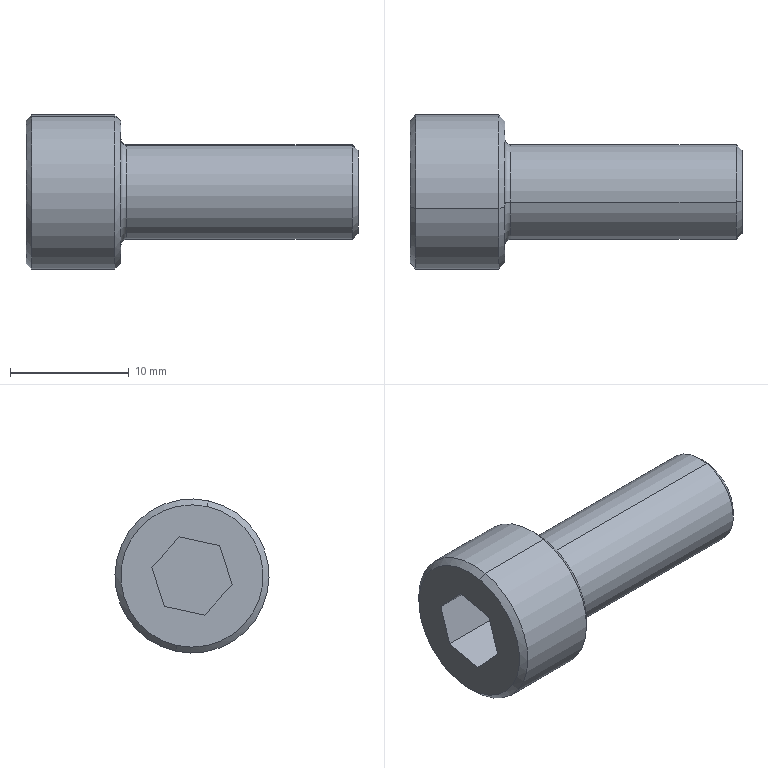Part | NX | features BREP 1 | 1 solid | 22 faces | box 28 x 13 x 13 mm | volume 1869 mm3 | plane 10 | cone 6 | cylinder 4 | torus 2 | commonest cylinder face diameters 8 x2 13 x2
STEP:
#1=CARTESIAN_POINT('',(-655.355,-109.755,15.547));
#2=VERTEX_POINT('',#1);
#3=CARTESIAN_POINT('',(-655.355,-111.682,24.338));
#4=VERTEX_POINT('',#3);
#5=CARTESIAN_POINT('',(-655.355,-110.718,19.942));
#6=DIRECTION('',(-1.,0.,0.));
#7=DIRECTION('',(0.,-0.2141,0.9768));
#8=AXIS2_PLACEMENT_3D('',#5,#6,#7);
#9=CIRCLE('',#8,4.5);
#10=EDGE_CURVE('',#2,#4,#9,.T.);
#11=ORIENTED_EDGE('',*,*,#10,.F.);
#12=CARTESIAN_POINT('',(-654.855,-109.862,16.035));
#13=VERTEX_POINT('',#12);
#14=CARTESIAN_POINT('',(-654.855,-109.755,15.547));
#15=DIRECTION('',(0.,0.9768,0.2141));
#16=DIRECTION('',(0.,0.2141,-0.9768));
#17=AXIS2_PLACEMENT_3D('',#14,#15,#16);
#18=CIRCLE('',#17,0.5);
#19=EDGE_CURVE('',#13,#2,#18,.F.);
#20=ORIENTED_EDGE('',*,*,#19,.F.);
#21=CARTESIAN_POINT('',(-654.855,-111.575,23.85));
#22=VERTEX_POINT('',#21);
#23=CARTESIAN_POINT('',(-654.855,-110.718,19.942));
#24=DIRECTION('',(1.,0.,0.));
#25=DIRECTION('',(0.,-0.2141,0.9768));
#26=AXIS2_PLACEMENT_3D('',#23,#24,#25);
#27=CIRCLE('',#26,4.);
#28=EDGE_CURVE('',#22,#13,#27,.T.);
#29=ORIENTED_EDGE('',*,*,#28,.F.);
#30=CARTESIAN_POINT('',(-654.855,-111.682,24.338));
#31=DIRECTION('',(0.,-0.9768,-0.2141));
#32=DIRECTION('',(1.,0.,0.));
#33=AXIS2_PLACEMENT_3D('',#30,#31,#32);
#34=CIRCLE('',#33,0.5);
#35=EDGE_CURVE('',#22,#4,#34,.F.);
#36=ORIENTED_EDGE('',*,*,#35,.T.);
#37=EDGE_LOOP('',(#11,#20,#29,#36));
#38=FACE_BOUND('',#37,.T.);
#39=CARTESIAN_POINT('',(-654.855,-110.718,19.942));
#40=DIRECTION('',(-1.,0.,0.));
#41=DIRECTION('',(0.,-0.2141,0.9768));
#42=AXIS2_PLACEMENT_3D('',#39,#40,#41);
#43=TOROIDAL_SURFACE('',#42,4.5,0.5);
#44=ADVANCED_FACE('',(#38),#43,.F.);
#45=CARTESIAN_POINT('',(-635.355,-109.969,16.524));
#46=VERTEX_POINT('',#45);
#47=CARTESIAN_POINT('',(-635.355,-111.468,23.361));
#48=VERTEX_POINT('',#47);
#49=CARTESIAN_POINT('',(-635.355,-110.718,19.942));
#50=DIRECTION('',(1.,0.,0.));
#51=DIRECTION('',(0.,-0.2141,0.9768));
#52=AXIS2_PLACEMENT_3D('',#49,#50,#51);
#53=CIRCLE('',#52,3.5);
#54=EDGE_CURVE('',#46,#48,#53,.T.);
#55=ORIENTED_EDGE('',*,*,#54,.F.);
#56=CARTESIAN_POINT('',(-635.855,-109.862,16.035));
#57=VERTEX_POINT('',#56);
#58=CARTESIAN_POINT('',(-635.855,-109.862,16.035));
#59=DIRECTION('',(-0.7071,0.1514,-0.6907));
#60=VECTOR('',#59,1000.);
#61=LINE('',#58,#60);
#62=EDGE_CURVE('',#57,#46,#61,.F.);
#63=ORIENTED_EDGE('',*,*,#62,.F.);
#64=CARTESIAN_POINT('',(-635.855,-111.575,23.85));
#65=VERTEX_POINT('',#64);
#66=CARTESIAN_POINT('',(-635.855,-110.718,19.942));
#67=DIRECTION('',(-1.,0.,0.));
#68=DIRECTION('',(0.,-0.2141,0.9768));
#69=AXIS2_PLACEMENT_3D('',#66,#67,#68);
#70=CIRCLE('',#69,4.);
#71=EDGE_CURVE('',#65,#57,#70,.T.);
#72=ORIENTED_EDGE('',*,*,#71,.F.);
#73=CARTESIAN_POINT('',(-635.855,-111.575,23.85));
#74=DIRECTION('',(-0.7071,-0.1514,0.6907));
#75=VECTOR('',#74,1000.);
#76=LINE('',#73,#75);
#77=EDGE_CURVE('',#65,#48,#76,.F.);
#78=ORIENTED_EDGE('',*,*,#77,.T.);
#79=EDGE_LOOP('',(#55,#63,#72,#78));
#80=FACE_BOUND('',#79,.T.);
#81=CARTESIAN_POINT('',(-635.855,-110.718,19.942));
#82=DIRECTION('',(-1.,0.,0.));
#83=DIRECTION('',(0.,-0.2141,0.9768));
#84=AXIS2_PLACEMENT_3D('',#81,#82,#83);
#85=CONICAL_SURFACE('',#84,4.,0.7854);
#86=ADVANCED_FACE('',(#80),#85,.T.);
#87=CARTESIAN_POINT('',(-663.355,-112.003,25.803));
#88=VERTEX_POINT('',#87);
#89=CARTESIAN_POINT('',(-663.355,-109.434,14.082));
#90=VERTEX_POINT('',#89);
#91=CARTESIAN_POINT('',(-663.355,-110.718,19.942));
#92=DIRECTION('',(-1.,0.,0.));
#93=DIRECTION('',(0.,-0.2141,0.9768));
#94=AXIS2_PLACEMENT_3D('',#91,#92,#93);
#95=CIRCLE('',#94,6.);
#96=EDGE_CURVE('',#88,#90,#95,.T.);
#97=ORIENTED_EDGE('',*,*,#96,.F.);
#98=CARTESIAN_POINT('',(-662.855,-112.11,26.292));
#99=VERTEX_POINT('',#98);
#100=CARTESIAN_POINT('',(-663.355,-112.003,25.803));
#101=DIRECTION('',(0.7071,-0.1514,0.6907));
#102=VECTOR('',#101,1000.);
#103=LINE('',#100,#102);
#104=EDGE_CURVE('',#88,#99,#103,.T.);
#105=ORIENTED_EDGE('',*,*,#104,.T.);
#106=CARTESIAN_POINT('',(-662.855,-109.326,13.593));
#107=VERTEX_POINT('',#106);
#108=CARTESIAN_POINT('',(-662.855,-110.718,19.942));
#109=DIRECTION('',(1.,0.,0.));
#110=DIRECTION('',(0.,-0.2141,0.9768));
#111=AXIS2_PLACEMENT_3D('',#108,#109,#110);
#112=CIRCLE('',#111,6.5);
#113=EDGE_CURVE('',#107,#99,#112,.T.);
#114=ORIENTED_EDGE('',*,*,#113,.F.);
#115=CARTESIAN_POINT('',(-663.355,-109.434,14.082));
#116=DIRECTION('',(0.7071,0.1514,-0.6907));
#117=VECTOR('',#116,1000.);
#118=LINE('',#115,#117);
#119=EDGE_CURVE('',#90,#107,#118,.T.);
#120=ORIENTED_EDGE('',*,*,#119,.F.);
#121=EDGE_LOOP('',(#97,#105,#114,#120));
#122=FACE_BOUND('',#121,.T.);
#123=CARTESIAN_POINT('',(-663.355,-110.718,19.942));
#124=DIRECTION('',(1.,0.,0.));
#125=DIRECTION('',(0.,0.2141,-0.9768));
#126=AXIS2_PLACEMENT_3D('',#123,#124,#125);
#127=CONICAL_SURFACE('',#126,6.,0.7854);
#128=ADVANCED_FACE('',(#122),#127,.T.);
#129=CARTESIAN_POINT('',(-655.355,-109.434,14.082));
#130=VERTEX_POINT('',#129);
#131=CARTESIAN_POINT('',(-655.355,-112.003,25.803));
#132=VERTEX_POINT('',#131);
#133=CARTESIAN_POINT('',(-655.355,-110.718,19.942));
#134=DIRECTION('',(1.,0.,0.));
#135=DIRECTION('',(0.,-0.2141,0.9768));
#136=AXIS2_PLACEMENT_3D('',#133,#134,#135);
#137=CIRCLE('',#136,6.);
#138=EDGE_CURVE('',#130,#132,#137,.T.);
#139=ORIENTED_EDGE('',*,*,#138,.F.);
#140=CARTESIAN_POINT('',(-655.855,-109.326,13.593));
#141=VERTEX_POINT('',#140);
#142=CARTESIAN_POINT('',(-655.855,-109.326,13.593));
#143=DIRECTION('',(-0.7071,0.1514,-0.6907));
#144=VECTOR('',#143,1000.);
#145=LINE('',#142,#144);
#146=EDGE_CURVE('',#141,#130,#145,.F.);
#147=ORIENTED_EDGE('',*,*,#146,.F.);
#148=CARTESIAN_POINT('',(-655.855,-112.11,26.292));
#149=VERTEX_POINT('',#148);
#150=CARTESIAN_POINT('',(-655.855,-110.718,19.942));
#151=DIRECTION('',(-1.,0.,0.));
#152=DIRECTION('',(0.,-0.2141,0.9768));
#153=AXIS2_PLACEMENT_3D('',#150,#151,#152);
#154=CIRCLE('',#153,6.5);
#155=EDGE_CURVE('',#149,#141,#154,.T.);
#156=ORIENTED_EDGE('',*,*,#155,.F.);
#157=CARTESIAN_POINT('',(-655.855,-112.11,26.292));
#158=DIRECTION('',(-0.7071,-0.1514,0.6907));
#159=VECTOR('',#158,1000.);
#160=LINE('',#157,#159);
#161=EDGE_CURVE('',#149,#132,#160,.F.);
#162=ORIENTED_EDGE('',*,*,#161,.T.);
#163=EDGE_LOOP('',(#139,#147,#156,#162));
#164=FACE_BOUND('',#163,.T.);
#165=CARTESIAN_POINT('',(-655.855,-110.718,19.942));
#166=DIRECTION('',(-1.,0.,0.));
#167=DIRECTION('',(0.,-0.2141,0.9768));
#168=AXIS2_PLACEMENT_3D('',#165,#166,#167);
#169=CONICAL_SURFACE('',#168,6.5,0.7854);
#170=ADVANCED_FACE('',(#164),#169,.T.);
#171=ORIENTED_EDGE('',*,*,#113,.T.);
#172=CARTESIAN_POINT('',(-663.355,-112.11,26.292));
#173=DIRECTION('',(1.,0.,0.));
#174=VECTOR('',#173,1000.);
#175=LINE('',#172,#174);
#176=EDGE_CURVE('',#99,#149,#175,.T.);
#177=ORIENTED_EDGE('',*,*,#176,.T.);
#178=ORIENTED_EDGE('',*,*,#155,.T.);
#179=CARTESIAN_POINT('',(-663.355,-109.326,13.593));
#180=DIRECTION('',(1.,0.,0.));
#181=VECTOR('',#180,1000.);
#182=LINE('',#179,#181);
#183=EDGE_CURVE('',#107,#141,#182,.T.);
#184=ORIENTED_EDGE('',*,*,#183,.F.);
#185=EDGE_LOOP('',(#171,#177,#178,#184));
#186=FACE_BOUND('',#185,.T.);
#187=CARTESIAN_POINT('',(-663.355,-110.718,19.942));
#188=DIRECTION('',(1.,0.,0.));
#189=DIRECTION('',(0.,0.2141,-0.9768));
#190=AXIS2_PLACEMENT_3D('',#187,#188,#189);
#191=CYLINDRICAL_SURFACE('',#190,6.5);
#192=ADVANCED_FACE('',(#186),#191,.T.);
#193=CARTESIAN_POINT('',(-654.855,-110.718,19.942));
#194=DIRECTION('',(1.,0.,0.));
#195=DIRECTION('',(0.,-0.2141,0.9768));
#196=AXIS2_PLACEMENT_3D('',#193,#194,#195);
#197=CIRCLE('',#196,4.);
#198=EDGE_CURVE('',#13,#22,#197,.T.);
#199=ORIENTED_EDGE('',*,*,#198,.T.);
#200=CARTESIAN_POINT('',(-655.355,-111.575,23.85));
#201=DIRECTION('',(1.,0.,0.));
#202=VECTOR('',#201,1000.);
#203=LINE('',#200,#202);
#204=EDGE_CURVE('',#22,#65,#203,.T.);
#205=ORIENTED_EDGE('',*,*,#204,.T.);
#206=ORIENTED_EDGE('',*,*,#71,.T.);
#207=CARTESIAN_POINT('',(-655.355,-109.862,16.035));
#208=DIRECTION('',(1.,0.,0.));
#209=VECTOR('',#208,1000.);
#210=LINE('',#207,#209);
#211=EDGE_CURVE('',#13,#57,#210,.T.);
#212=ORIENTED_EDGE('',*,*,#211,.F.);
#213=EDGE_LOOP('',(#199,#205,#206,#212));
#214=FACE_BOUND('',#213,.T.);
#215=CARTESIAN_POINT('',(-655.355,-110.718,19.942));
#216=DIRECTION('',(1.,0.,0.));
#217=DIRECTION('',(0.,0.2141,-0.9768));
#218=AXIS2_PLACEMENT_3D('',#215,#216,#217);
#219=CYLINDRICAL_SURFACE('',#218,4.);
#220=ADVANCED_FACE('',(#214),#219,.T.);
#221=ORIENTED_EDGE('',*,*,#204,.F.);
#222=ORIENTED_EDGE('',*,*,#28,.T.);
#223=ORIENTED_EDGE('',*,*,#211,.T.);
#224=CARTESIAN_POINT('',(-635.855,-110.718,19.942));
#225=DIRECTION('',(-1.,0.,0.));
#226=DIRECTION('',(0.,-0.2141,0.9768));
#227=AXIS2_PLACEMENT_3D('',#224,#225,#226);
#228=CIRCLE('',#227,4.);
#229=EDGE_CURVE('',#57,#65,#228,.T.);
#230=ORIENTED_EDGE('',*,*,#229,.T.);
#231=EDGE_LOOP('',(#221,#222,#223,#230));
#232=FACE_BOUND('',#231,.T.);
#233=CARTESIAN_POINT('',(-655.355,-110.718,19.942));
#234=DIRECTION('',(1.,0.,0.));
#235=DIRECTION('',(0.,0.2141,-0.9768));
#236=AXIS2_PLACEMENT_3D('',#233,#234,#235);
#237=CYLINDRICAL_SURFACE('',#236,4.);
#238=ADVANCED_FACE('',(#232),#237,.T.);
#239=CARTESIAN_POINT('',(-635.355,-110.718,19.942));
#240=DIRECTION('',(1.,0.,0.));
#241=DIRECTION('',(0.,-0.2141,0.9768));
#242=AXIS2_PLACEMENT_3D('',#239,#240,#241);
#243=CIRCLE('',#242,3.5);
#244=EDGE_CURVE('',#48,#46,#243,.T.);
#245=ORIENTED_EDGE('',*,*,#244,.T.);
#246=ORIENTED_EDGE('',*,*,#54,.T.);
#247=EDGE_LOOP('',(#245,#246));
#248=FACE_BOUND('',#247,.T.);
#249=CARTESIAN_POINT('',(-635.355,-110.718,19.942));
#250=DIRECTION('',(-1.,0.,0.));
#251=DIRECTION('',(0.,-0.2141,0.9768));
#252=AXIS2_PLACEMENT_3D('',#249,#250,#251);
#253=PLANE('',#252);
#254=ADVANCED_FACE('',(#248),#253,.F.);
#255=ORIENTED_EDGE('',*,*,#176,.F.);
#256=CARTESIAN_POINT('',(-662.855,-110.718,19.942));
#257=DIRECTION('',(1.,0.,0.));
#258=DIRECTION('',(0.,-0.2141,0.9768));
#259=AXIS2_PLACEMENT_3D('',#256,#257,#258);
#260=CIRCLE('',#259,6.5);
#261=EDGE_CURVE('',#99,#107,#260,.T.);
#262=ORIENTED_EDGE('',*,*,#261,.T.);
#263=ORIENTED_EDGE('',*,*,#183,.T.);
#264=CARTESIAN_POINT('',(-655.855,-110.718,19.942));
#265=DIRECTION('',(-1.,0.,0.));
#266=DIRECTION('',(0.,-0.2141,0.9768));
#267=AXIS2_PLACEMENT_3D('',#264,#265,#266);
#268=CIRCLE('',#267,6.5);
#269=EDGE_CURVE('',#141,#149,#268,.T.);
#270=ORIENTED_EDGE('',*,*,#269,.T.);
#271=EDGE_LOOP('',(#255,#262,#263,#270));
#272=FACE_BOUND('',#271,.T.);
#273=CARTESIAN_POINT('',(-663.355,-110.718,19.942));
#274=DIRECTION('',(1.,0.,0.));
#275=DIRECTION('',(0.,0.2141,-0.9768));
#276=AXIS2_PLACEMENT_3D('',#273,#274,#275);
#277=CYLINDRICAL_SURFACE('',#276,6.5);
#278=ADVANCED_FACE('',(#272),#277,.T.);
#279=CARTESIAN_POINT('',(-663.355,-110.718,19.942));
#280=DIRECTION('',(-1.,0.,0.));
#281=DIRECTION('',(0.,-0.2141,0.9768));
#282=AXIS2_PLACEMENT_3D('',#279,#280,#281);
#283=CIRCLE('',#282,6.);
#284=EDGE_CURVE('',#90,#88,#283,.T.);
#285=ORIENTED_EDGE('',*,*,#284,.T.);
#286=ORIENTED_EDGE('',*,*,#96,.T.);
#287=EDGE_LOOP('',(#285,#286));
#288=FACE_BOUND('',#287,.T.);
#289=CARTESIAN_POINT('',(-663.355,-109.669,23.244));
#290=VERTEX_POINT('',#289);
#291=CARTESIAN_POINT('',(-663.355,-107.335,20.684));
#292=VERTEX_POINT('',#291);
#293=CARTESIAN_POINT('',(-663.355,-109.669,23.244));
#294=DIRECTION('',(0.,0.6738,-0.7389));
#295=VECTOR('',#294,1000.);
#296=LINE('',#293,#295);
#297=EDGE_CURVE('',#290,#292,#296,.T.);
#298=ORIENTED_EDGE('',*,*,#297,.F.);
#299=CARTESIAN_POINT('',(-663.355,-113.053,22.502));
#300=VERTEX_POINT('',#299);
#301=CARTESIAN_POINT('',(-663.355,-113.053,22.502));
#302=DIRECTION('',(0.,0.9768,0.2141));
#303=VECTOR('',#302,1000.);
#304=LINE('',#301,#303);
#305=EDGE_CURVE('',#300,#290,#304,.T.);
#306=ORIENTED_EDGE('',*,*,#305,.F.);
#307=CARTESIAN_POINT('',(-663.355,-114.102,19.201));
#308=VERTEX_POINT('',#307);
#309=CARTESIAN_POINT('',(-663.355,-114.102,19.201));
#310=DIRECTION('',(0.,0.303,0.953));
#311=VECTOR('',#310,1000.);
#312=LINE('',#309,#311);
#313=EDGE_CURVE('',#308,#300,#312,.T.);
#314=ORIENTED_EDGE('',*,*,#313,.F.);
#315=CARTESIAN_POINT('',(-663.355,-111.768,16.641));
#316=VERTEX_POINT('',#315);
#317=CARTESIAN_POINT('',(-663.355,-111.768,16.641));
#318=DIRECTION('',(0.,-0.6738,0.7389));
#319=VECTOR('',#318,1000.);
#320=LINE('',#317,#319);
#321=EDGE_CURVE('',#316,#308,#320,.T.);
#322=ORIENTED_EDGE('',*,*,#321,.F.);
#323=CARTESIAN_POINT('',(-663.355,-108.384,17.383));
#324=VERTEX_POINT('',#323);
#325=CARTESIAN_POINT('',(-663.355,-108.384,17.383));
#326=DIRECTION('',(0.,-0.9768,-0.2141));
#327=VECTOR('',#326,1000.);
#328=LINE('',#325,#327);
#329=EDGE_CURVE('',#324,#316,#328,.T.);
#330=ORIENTED_EDGE('',*,*,#329,.F.);
#331=CARTESIAN_POINT('',(-663.355,-107.335,20.684));
#332=DIRECTION('',(0.,-0.303,-0.953));
#333=VECTOR('',#332,1000.);
#334=LINE('',#331,#333);
#335=EDGE_CURVE('',#292,#324,#334,.T.);
#336=ORIENTED_EDGE('',*,*,#335,.F.);
#337=EDGE_LOOP('',(#298,#306,#314,#322,#330,#336));
#338=FACE_BOUND('',#337,.T.);
#339=CARTESIAN_POINT('',(-663.355,-110.718,19.942));
#340=DIRECTION('',(-1.,0.,0.));
#341=DIRECTION('',(0.,-0.2141,0.9768));
#342=AXIS2_PLACEMENT_3D('',#339,#340,#341);
#343=PLANE('',#342);
#344=ADVANCED_FACE('',(#288,#338),#343,.T.);
#345=CARTESIAN_POINT('',(-655.355,-110.718,19.942));
#346=DIRECTION('',(-1.,0.,0.));
#347=DIRECTION('',(0.,-0.2141,0.9768));
#348=AXIS2_PLACEMENT_3D('',#345,#346,#347);
#349=CIRCLE('',#348,4.5);
#350=EDGE_CURVE('',#4,#2,#349,.T.);
#351=ORIENTED_EDGE('',*,*,#350,.T.);
#352=ORIENTED_EDGE('',*,*,#10,.T.);
#353=EDGE_LOOP('',(#351,#352));
#354=FACE_BOUND('',#353,.T.);
#355=CARTESIAN_POINT('',(-655.355,-110.718,19.942));
#356=DIRECTION('',(1.,0.,0.));
#357=DIRECTION('',(0.,-0.2141,0.9768));
#358=AXIS2_PLACEMENT_3D('',#355,#356,#357);
#359=CIRCLE('',#358,6.);
#360=EDGE_CURVE('',#132,#130,#359,.T.);
#361=ORIENTED_EDGE('',*,*,#360,.T.);
#362=ORIENTED_EDGE('',*,*,#138,.T.);
#363=EDGE_LOOP('',(#361,#362));
#364=FACE_BOUND('',#363,.T.);
#365=CARTESIAN_POINT('',(-655.355,-110.718,19.942));
#366=DIRECTION('',(-1.,0.,0.));
#367=DIRECTION('',(0.,-0.2141,0.9768));
#368=AXIS2_PLACEMENT_3D('',#365,#366,#367);
#369=PLANE('',#368);
#370=ADVANCED_FACE('',(#354,#364),#369,.F.);
#371=ORIENTED_EDGE('',*,*,#297,.T.);
#372=CARTESIAN_POINT('',(-657.355,-107.335,20.684));
#373=VERTEX_POINT('',#372);
#374=CARTESIAN_POINT('',(-657.355,-107.335,20.684));
#375=DIRECTION('',(-1.,0.,0.));
#376=VECTOR('',#375,1000.);
#377=LINE('',#374,#376);
#378=EDGE_CURVE('',#373,#292,#377,.T.);
#379=ORIENTED_EDGE('',*,*,#378,.F.);
#380=CARTESIAN_POINT('',(-657.355,-109.669,23.244));
#381=VERTEX_POINT('',#380);
#382=CARTESIAN_POINT('',(-657.355,-109.669,23.244));
#383=DIRECTION('',(0.,0.6738,-0.7389));
#384=VECTOR('',#383,1000.);
#385=LINE('',#382,#384);
#386=EDGE_CURVE('',#381,#373,#385,.T.);
#387=ORIENTED_EDGE('',*,*,#386,.F.);
#388=CARTESIAN_POINT('',(-657.355,-109.669,23.244));
#389=DIRECTION('',(-1.,0.,0.));
#390=VECTOR('',#389,1000.);
#391=LINE('',#388,#390);
#392=EDGE_CURVE('',#381,#290,#391,.T.);
#393=ORIENTED_EDGE('',*,*,#392,.T.);
#394=EDGE_LOOP('',(#371,#379,#387,#393));
#395=FACE_BOUND('',#394,.T.);
#396=CARTESIAN_POINT('',(-657.355,-109.669,23.244));
#397=DIRECTION('',(0.,0.7389,0.6738));
#398=DIRECTION('',(0.,0.6738,-0.7389));
#399=AXIS2_PLACEMENT_3D('',#396,#397,#398);
#400=PLANE('',#399);
#401=ADVANCED_FACE('',(#395),#400,.F.);
#402=ORIENTED_EDGE('',*,*,#305,.T.);
#403=ORIENTED_EDGE('',*,*,#392,.F.);
#404=CARTESIAN_POINT('',(-657.355,-113.053,22.502));
#405=VERTEX_POINT('',#404);
#406=CARTESIAN_POINT('',(-657.355,-113.053,22.502));
#407=DIRECTION('',(0.,0.9768,0.2141));
#408=VECTOR('',#407,1000.);
#409=LINE('',#406,#408);
#410=EDGE_CURVE('',#405,#381,#409,.T.);
#411=ORIENTED_EDGE('',*,*,#410,.F.);
#412=CARTESIAN_POINT('',(-657.355,-113.053,22.502));
#413=DIRECTION('',(-1.,0.,0.));
#414=VECTOR('',#413,1000.);
#415=LINE('',#412,#414);
#416=EDGE_CURVE('',#405,#300,#415,.T.);
#417=ORIENTED_EDGE('',*,*,#416,.T.);
#418=EDGE_LOOP('',(#402,#403,#411,#417));
#419=FACE_BOUND('',#418,.T.);
#420=CARTESIAN_POINT('',(-657.355,-113.053,22.502));
#421=DIRECTION('',(0.,-0.2141,0.9768));
#422=DIRECTION('',(0.,0.9768,0.2141));
#423=AXIS2_PLACEMENT_3D('',#420,#421,#422);
#424=PLANE('',#423);
#425=ADVANCED_FACE('',(#419),#424,.F.);
#426=ORIENTED_EDGE('',*,*,#313,.T.);
#427=ORIENTED_EDGE('',*,*,#416,.F.);
#428=CARTESIAN_POINT('',(-657.355,-114.102,19.201));
#429=VERTEX_POINT('',#428);
#430=CARTESIAN_POINT('',(-657.355,-114.102,19.201));
#431=DIRECTION('',(0.,0.303,0.953));
#432=VECTOR('',#431,1000.);
#433=LINE('',#430,#432);
#434=EDGE_CURVE('',#429,#405,#433,.T.);
#435=ORIENTED_EDGE('',*,*,#434,.F.);
#436=CARTESIAN_POINT('',(-657.355,-114.102,19.201));
#437=DIRECTION('',(-1.,0.,0.));
#438=VECTOR('',#437,1000.);
#439=LINE('',#436,#438);
#440=EDGE_CURVE('',#429,#308,#439,.T.);
#441=ORIENTED_EDGE('',*,*,#440,.T.);
#442=EDGE_LOOP('',(#426,#427,#435,#441));
#443=FACE_BOUND('',#442,.T.);
#444=CARTESIAN_POINT('',(-657.355,-114.102,19.201));
#445=DIRECTION('',(0.,-0.953,0.303));
#446=DIRECTION('',(0.,0.303,0.953));
#447=AXIS2_PLACEMENT_3D('',#444,#445,#446);
#448=PLANE('',#447);
#449=ADVANCED_FACE('',(#443),#448,.F.);
#450=ORIENTED_EDGE('',*,*,#321,.T.);
#451=ORIENTED_EDGE('',*,*,#440,.F.);
#452=CARTESIAN_POINT('',(-657.355,-111.768,16.641));
#453=VERTEX_POINT('',#452);
#454=CARTESIAN_POINT('',(-657.355,-111.768,16.641));
#455=DIRECTION('',(0.,-0.6738,0.7389));
#456=VECTOR('',#455,1000.);
#457=LINE('',#454,#456);
#458=EDGE_CURVE('',#453,#429,#457,.T.);
#459=ORIENTED_EDGE('',*,*,#458,.F.);
#460=CARTESIAN_POINT('',(-657.355,-111.768,16.641));
#461=DIRECTION('',(-1.,0.,0.));
#462=VECTOR('',#461,1000.);
#463=LINE('',#460,#462);
#464=EDGE_CURVE('',#453,#316,#463,.T.);
#465=ORIENTED_EDGE('',*,*,#464,.T.);
#466=EDGE_LOOP('',(#450,#451,#459,#465));
#467=FACE_BOUND('',#466,.T.);
#468=CARTESIAN_POINT('',(-657.355,-111.768,16.641));
#469=DIRECTION('',(0.,-0.7389,-0.6738));
#470=DIRECTION('',(0.,-0.6738,0.7389));
#471=AXIS2_PLACEMENT_3D('',#468,#469,#470);
#472=PLANE('',#471);
#473=ADVANCED_FACE('',(#467),#472,.F.);
#474=ORIENTED_EDGE('',*,*,#329,.T.);
#475=ORIENTED_EDGE('',*,*,#464,.F.);
#476=CARTESIAN_POINT('',(-657.355,-108.384,17.383));
#477=VERTEX_POINT('',#476);
#478=CARTESIAN_POINT('',(-657.355,-108.384,17.383));
#479=DIRECTION('',(0.,-0.9768,-0.2141));
#480=VECTOR('',#479,1000.);
#481=LINE('',#478,#480);
#482=EDGE_CURVE('',#477,#453,#481,.T.);
#483=ORIENTED_EDGE('',*,*,#482,.F.);
#484=CARTESIAN_POINT('',(-657.355,-108.384,17.383));
#485=DIRECTION('',(-1.,0.,0.));
#486=VECTOR('',#485,1000.);
#487=LINE('',#484,#486);
#488=EDGE_CURVE('',#477,#324,#487,.T.);
#489=ORIENTED_EDGE('',*,*,#488,.T.);
#490=EDGE_LOOP('',(#474,#475,#483,#489));
#491=FACE_BOUND('',#490,.T.);
#492=CARTESIAN_POINT('',(-657.355,-108.384,17.383));
#493=DIRECTION('',(0.,0.2141,-0.9768));
#494=DIRECTION('',(0.,-0.9768,-0.2141));
#495=AXIS2_PLACEMENT_3D('',#492,#493,#494);
#496=PLANE('',#495);
#497=ADVANCED_FACE('',(#491),#496,.F.);
#498=ORIENTED_EDGE('',*,*,#335,.T.);
#499=ORIENTED_EDGE('',*,*,#488,.F.);
#500=CARTESIAN_POINT('',(-657.355,-107.335,20.684));
#501=DIRECTION('',(0.,-0.303,-0.953));
#502=VECTOR('',#501,1000.);
#503=LINE('',#500,#502);
#504=EDGE_CURVE('',#373,#477,#503,.T.);
#505=ORIENTED_EDGE('',*,*,#504,.F.);
#506=ORIENTED_EDGE('',*,*,#378,.T.);
#507=EDGE_LOOP('',(#498,#499,#505,#506));
#508=FACE_BOUND('',#507,.T.);
#509=CARTESIAN_POINT('',(-657.355,-107.335,20.684));
#510=DIRECTION('',(0.,0.953,-0.303));
#511=DIRECTION('',(0.,-0.303,-0.953));
#512=AXIS2_PLACEMENT_3D('',#509,#510,#511);
#513=PLANE('',#512);
#514=ADVANCED_FACE('',(#508),#513,.F.);
#515=ORIENTED_EDGE('',*,*,#386,.T.);
#516=ORIENTED_EDGE('',*,*,#504,.T.);
#517=ORIENTED_EDGE('',*,*,#482,.T.);
#518=ORIENTED_EDGE('',*,*,#458,.T.);
#519=ORIENTED_EDGE('',*,*,#434,.T.);
#520=ORIENTED_EDGE('',*,*,#410,.T.);
#521=EDGE_LOOP('',(#515,#516,#517,#518,#519,#520));
#522=FACE_BOUND('',#521,.T.);
#523=CARTESIAN_POINT('',(-657.355,-110.718,19.942));
#524=DIRECTION('',(-1.,0.,0.));
#525=DIRECTION('',(0.,-0.2141,0.9768));
#526=AXIS2_PLACEMENT_3D('',#523,#524,#525);
#527=PLANE('',#526);
#528=ADVANCED_FACE('',(#522),#527,.T.);
#529=ORIENTED_EDGE('',*,*,#146,.T.);
#530=ORIENTED_EDGE('',*,*,#360,.F.);
#531=ORIENTED_EDGE('',*,*,#161,.F.);
#532=ORIENTED_EDGE('',*,*,#269,.F.);
#533=EDGE_LOOP('',(#529,#530,#531,#532));
#534=FACE_BOUND('',#533,.T.);
#535=CARTESIAN_POINT('',(-655.855,-110.718,19.942));
#536=DIRECTION('',(-1.,0.,0.));
#537=DIRECTION('',(0.,-0.2141,0.9768));
#538=AXIS2_PLACEMENT_3D('',#535,#536,#537);
#539=CONICAL_SURFACE('',#538,6.5,0.7854);
#540=ADVANCED_FACE('',(#534),#539,.T.);
#541=ORIENTED_EDGE('',*,*,#104,.F.);
#542=ORIENTED_EDGE('',*,*,#284,.F.);
#543=ORIENTED_EDGE('',*,*,#119,.T.);
#544=ORIENTED_EDGE('',*,*,#261,.F.);
#545=EDGE_LOOP('',(#541,#542,#543,#544));
#546=FACE_BOUND('',#545,.T.);
#547=CARTESIAN_POINT('',(-663.355,-110.718,19.942));
#548=DIRECTION('',(1.,0.,0.));
#549=DIRECTION('',(0.,0.2141,-0.9768));
#550=AXIS2_PLACEMENT_3D('',#547,#548,#549);
#551=CONICAL_SURFACE('',#550,6.,0.7854);
#552=ADVANCED_FACE('',(#546),#551,.T.);
#553=ORIENTED_EDGE('',*,*,#62,.T.);
#554=ORIENTED_EDGE('',*,*,#244,.F.);
#555=ORIENTED_EDGE('',*,*,#77,.F.);
#556=ORIENTED_EDGE('',*,*,#229,.F.);
#557=EDGE_LOOP('',(#553,#554,#555,#556));
#558=FACE_BOUND('',#557,.T.);
#559=CARTESIAN_POINT('',(-635.855,-110.718,19.942));
#560=DIRECTION('',(-1.,0.,0.));
#561=DIRECTION('',(0.,-0.2141,0.9768));
#562=AXIS2_PLACEMENT_3D('',#559,#560,#561);
#563=CONICAL_SURFACE('',#562,4.,0.7854);
#564=ADVANCED_FACE('',(#558),#563,.T.);
#565=ORIENTED_EDGE('',*,*,#19,.T.);
#566=ORIENTED_EDGE('',*,*,#350,.F.);
#567=ORIENTED_EDGE('',*,*,#35,.F.);
#568=ORIENTED_EDGE('',*,*,#198,.F.);
#569=EDGE_LOOP('',(#565,#566,#567,#568));
#570=FACE_BOUND('',#569,.T.);
#571=CARTESIAN_POINT('',(-654.855,-110.718,19.942));
#572=DIRECTION('',(-1.,0.,0.));
#573=DIRECTION('',(0.,-0.2141,0.9768));
#574=AXIS2_PLACEMENT_3D('',#571,#572,#573);
#575=TOROIDAL_SURFACE('',#574,4.5,0.5);
#576=ADVANCED_FACE('',(#570),#575,.F.);
#577=CLOSED_SHELL('',(#44,#86,#128,#170,#192,#220,#238,#254,#278,#344,#370,#401,#425,#449,#473,#497,#514,#528,#540,#552,#564,#576));
#578=MANIFOLD_SOLID_BREP('',#577);
#579=(LENGTH_UNIT()NAMED_UNIT(*)SI_UNIT(.MILLI.,.METRE.));
#580=UNCERTAINTY_MEASURE_WITH_UNIT(LENGTH_MEASURE(0.00001),#579,'','');
#581=(NAMED_UNIT(*)PLANE_ANGLE_UNIT()SI_UNIT($,.RADIAN.));
#582=(NAMED_UNIT(*)SI_UNIT($,.STERADIAN.)SOLID_ANGLE_UNIT());
#583=(GEOMETRIC_REPRESENTATION_CONTEXT(3)GLOBAL_UNCERTAINTY_ASSIGNED_CONTEXT((#580))GLOBAL_UNIT_ASSIGNED_CONTEXT((#579,#581,#582))REPRESENTATION_CONTEXT('',''));
#584=ADVANCED_BREP_SHAPE_REPRESENTATION('',(#578),#583);